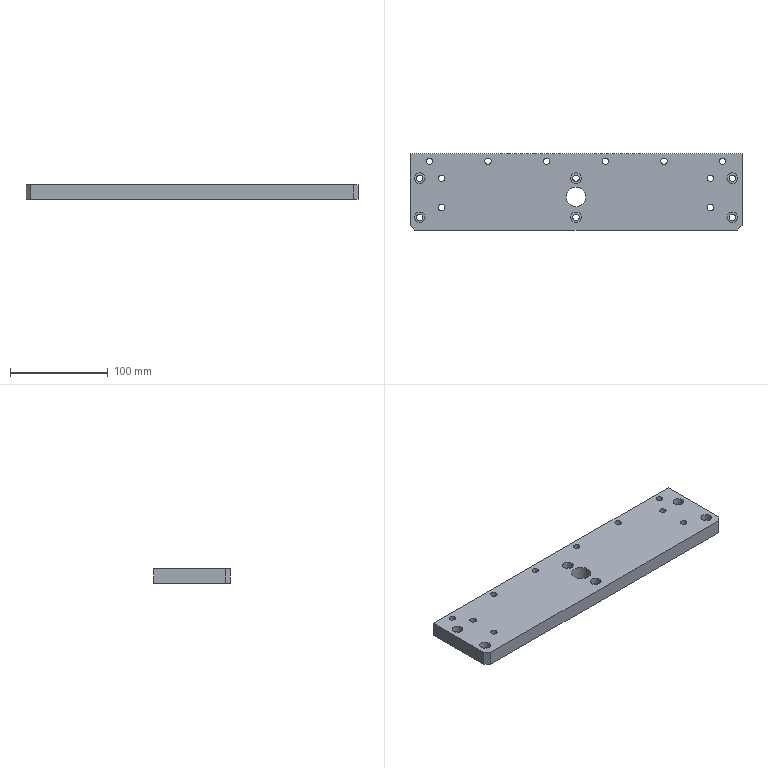Part | NX | 1 solid | 57 faces | box 340 x 78 x 15 mm | volume 377884 mm3 | cylinder 33 | plane 24 | commonest cylinder face diameters 6.6 x16 11 x16 20 x1
STEP:
#1=CARTESIAN_POINT('',(170.,-34.,7.5));
#2=VERTEX_POINT('',#1);
#3=CARTESIAN_POINT('',(170.,39.,7.5));
#4=VERTEX_POINT('',#3);
#5=CARTESIAN_POINT('',(170.,39.,7.5));
#6=DIRECTION('',(0.,1.,0.));
#7=VECTOR('',#6,1000.);
#8=LINE('',#5,#7);
#9=EDGE_CURVE('',#2,#4,#8,.T.);
#10=ORIENTED_EDGE('',*,*,#9,.F.);
#11=CARTESIAN_POINT('',(170.,-34.,-7.5));
#12=VERTEX_POINT('',#11);
#13=CARTESIAN_POINT('',(170.,-34.,7.5));
#14=DIRECTION('',(0.,0.,-1.));
#15=VECTOR('',#14,1000.);
#16=LINE('',#13,#15);
#17=EDGE_CURVE('',#2,#12,#16,.T.);
#18=ORIENTED_EDGE('',*,*,#17,.T.);
#19=CARTESIAN_POINT('',(170.,39.,-7.5));
#20=VERTEX_POINT('',#19);
#21=CARTESIAN_POINT('',(170.,39.,-7.5));
#22=DIRECTION('',(0.,1.,0.));
#23=VECTOR('',#22,1000.);
#24=LINE('',#21,#23);
#25=EDGE_CURVE('',#12,#20,#24,.T.);
#26=ORIENTED_EDGE('',*,*,#25,.T.);
#27=CARTESIAN_POINT('',(170.,39.,7.5));
#28=DIRECTION('',(0.,0.,-1.));
#29=VECTOR('',#28,1000.);
#30=LINE('',#27,#29);
#31=EDGE_CURVE('',#4,#20,#30,.T.);
#32=ORIENTED_EDGE('',*,*,#31,.F.);
#33=EDGE_LOOP('',(#10,#18,#26,#32));
#34=FACE_BOUND('',#33,.T.);
#35=CARTESIAN_POINT('',(170.,39.,7.5));
#36=DIRECTION('',(-1.,0.,0.));
#37=DIRECTION('',(0.,-1.,0.));
#38=AXIS2_PLACEMENT_3D('',#35,#36,#37);
#39=PLANE('',#38);
#40=ADVANCED_FACE('',(#34),#39,.F.);
#41=CARTESIAN_POINT('',(-170.,39.,-7.5));
#42=VERTEX_POINT('',#41);
#43=CARTESIAN_POINT('',(-170.,39.,-7.5));
#44=DIRECTION('',(-1.,0.,0.));
#45=VECTOR('',#44,1000.);
#46=LINE('',#43,#45);
#47=EDGE_CURVE('',#20,#42,#46,.T.);
#48=ORIENTED_EDGE('',*,*,#47,.T.);
#49=CARTESIAN_POINT('',(-170.,39.,7.5));
#50=VERTEX_POINT('',#49);
#51=CARTESIAN_POINT('',(-170.,39.,7.5));
#52=DIRECTION('',(0.,0.,-1.));
#53=VECTOR('',#52,1000.);
#54=LINE('',#51,#53);
#55=EDGE_CURVE('',#50,#42,#54,.T.);
#56=ORIENTED_EDGE('',*,*,#55,.F.);
#57=CARTESIAN_POINT('',(-170.,39.,7.5));
#58=DIRECTION('',(-1.,0.,0.));
#59=VECTOR('',#58,1000.);
#60=LINE('',#57,#59);
#61=EDGE_CURVE('',#4,#50,#60,.T.);
#62=ORIENTED_EDGE('',*,*,#61,.F.);
#63=ORIENTED_EDGE('',*,*,#31,.T.);
#64=EDGE_LOOP('',(#48,#56,#62,#63));
#65=FACE_BOUND('',#64,.T.);
#66=CARTESIAN_POINT('',(-170.,39.,7.5));
#67=DIRECTION('',(0.,-1.,0.));
#68=DIRECTION('',(0.,0.,-1.));
#69=AXIS2_PLACEMENT_3D('',#66,#67,#68);
#70=PLANE('',#69);
#71=ADVANCED_FACE('',(#65),#70,.F.);
#72=CARTESIAN_POINT('',(-170.,-34.,-7.5));
#73=VERTEX_POINT('',#72);
#74=CARTESIAN_POINT('',(-170.,39.,-7.5));
#75=DIRECTION('',(0.,-1.,0.));
#76=VECTOR('',#75,1000.);
#77=LINE('',#74,#76);
#78=EDGE_CURVE('',#42,#73,#77,.T.);
#79=ORIENTED_EDGE('',*,*,#78,.T.);
#80=CARTESIAN_POINT('',(-170.,-34.,7.5));
#81=VERTEX_POINT('',#80);
#82=CARTESIAN_POINT('',(-170.,-34.,7.5));
#83=DIRECTION('',(0.,0.,1.));
#84=VECTOR('',#83,1000.);
#85=LINE('',#82,#84);
#86=EDGE_CURVE('',#73,#81,#85,.T.);
#87=ORIENTED_EDGE('',*,*,#86,.T.);
#88=CARTESIAN_POINT('',(-170.,39.,7.5));
#89=DIRECTION('',(0.,-1.,0.));
#90=VECTOR('',#89,1000.);
#91=LINE('',#88,#90);
#92=EDGE_CURVE('',#50,#81,#91,.T.);
#93=ORIENTED_EDGE('',*,*,#92,.F.);
#94=ORIENTED_EDGE('',*,*,#55,.T.);
#95=EDGE_LOOP('',(#79,#87,#93,#94));
#96=FACE_BOUND('',#95,.T.);
#97=CARTESIAN_POINT('',(-170.,39.,7.5));
#98=DIRECTION('',(1.,0.,0.));
#99=DIRECTION('',(0.,0.,-1.));
#100=AXIS2_PLACEMENT_3D('',#97,#98,#99);
#101=PLANE('',#100);
#102=ADVANCED_FACE('',(#96),#101,.F.);
#103=CARTESIAN_POINT('',(-165.,-39.,-7.5));
#104=VERTEX_POINT('',#103);
#105=CARTESIAN_POINT('',(165.,-39.,-7.5));
#106=VERTEX_POINT('',#105);
#107=CARTESIAN_POINT('',(-170.,-39.,-7.5));
#108=DIRECTION('',(1.,0.,0.));
#109=VECTOR('',#108,1000.);
#110=LINE('',#107,#109);
#111=EDGE_CURVE('',#104,#106,#110,.T.);
#112=ORIENTED_EDGE('',*,*,#111,.T.);
#113=CARTESIAN_POINT('',(165.,-39.,7.5));
#114=VERTEX_POINT('',#113);
#115=CARTESIAN_POINT('',(165.,-39.,7.5));
#116=DIRECTION('',(0.,0.,1.));
#117=VECTOR('',#116,1000.);
#118=LINE('',#115,#117);
#119=EDGE_CURVE('',#106,#114,#118,.T.);
#120=ORIENTED_EDGE('',*,*,#119,.T.);
#121=CARTESIAN_POINT('',(-165.,-39.,7.5));
#122=VERTEX_POINT('',#121);
#123=CARTESIAN_POINT('',(-170.,-39.,7.5));
#124=DIRECTION('',(1.,0.,0.));
#125=VECTOR('',#124,1000.);
#126=LINE('',#123,#125);
#127=EDGE_CURVE('',#122,#114,#126,.T.);
#128=ORIENTED_EDGE('',*,*,#127,.F.);
#129=CARTESIAN_POINT('',(-165.,-39.,7.5));
#130=DIRECTION('',(0.,0.,-1.));
#131=VECTOR('',#130,1000.);
#132=LINE('',#129,#131);
#133=EDGE_CURVE('',#122,#104,#132,.T.);
#134=ORIENTED_EDGE('',*,*,#133,.T.);
#135=EDGE_LOOP('',(#112,#120,#128,#134));
#136=FACE_BOUND('',#135,.T.);
#137=CARTESIAN_POINT('',(-170.,-39.,7.5));
#138=DIRECTION('',(0.,1.,0.));
#139=DIRECTION('',(0.,0.,1.));
#140=AXIS2_PLACEMENT_3D('',#137,#138,#139);
#141=PLANE('',#140);
#142=ADVANCED_FACE('',(#136),#141,.F.);
#143=CARTESIAN_POINT('',(10.,-5.,7.5));
#144=VERTEX_POINT('',#143);
#145=CARTESIAN_POINT('',(0.,-5.,7.5));
#146=DIRECTION('',(0.,0.,1.));
#147=DIRECTION('',(1.,0.,0.));
#148=AXIS2_PLACEMENT_3D('',#145,#146,#147);
#149=CIRCLE('',#148,10.);
#150=EDGE_CURVE('',#144,#144,#149,.T.);
#151=ORIENTED_EDGE('',*,*,#150,.F.);
#152=EDGE_LOOP('',(#151));
#153=FACE_BOUND('',#152,.T.);
#154=CARTESIAN_POINT('',(165.5,-26.,7.5));
#155=VERTEX_POINT('',#154);
#156=CARTESIAN_POINT('',(160.,-26.,7.5));
#157=DIRECTION('',(0.,0.,1.));
#158=DIRECTION('',(1.,0.,0.));
#159=AXIS2_PLACEMENT_3D('',#156,#157,#158);
#160=CIRCLE('',#159,5.5);
#161=EDGE_CURVE('',#155,#155,#160,.T.);
#162=ORIENTED_EDGE('',*,*,#161,.F.);
#163=EDGE_LOOP('',(#162));
#164=FACE_BOUND('',#163,.T.);
#165=CARTESIAN_POINT('',(5.5,-26.,7.5));
#166=VERTEX_POINT('',#165);
#167=CARTESIAN_POINT('',(0.,-26.,7.5));
#168=DIRECTION('',(0.,0.,1.));
#169=DIRECTION('',(1.,0.,0.));
#170=AXIS2_PLACEMENT_3D('',#167,#168,#169);
#171=CIRCLE('',#170,5.5);
#172=EDGE_CURVE('',#166,#166,#171,.T.);
#173=ORIENTED_EDGE('',*,*,#172,.F.);
#174=EDGE_LOOP('',(#173));
#175=FACE_BOUND('',#174,.T.);
#176=CARTESIAN_POINT('',(-154.5,-26.,7.5));
#177=VERTEX_POINT('',#176);
#178=CARTESIAN_POINT('',(-160.,-26.,7.5));
#179=DIRECTION('',(0.,0.,1.));
#180=DIRECTION('',(1.,0.,0.));
#181=AXIS2_PLACEMENT_3D('',#178,#179,#180);
#182=CIRCLE('',#181,5.5);
#183=EDGE_CURVE('',#177,#177,#182,.T.);
#184=ORIENTED_EDGE('',*,*,#183,.F.);
#185=EDGE_LOOP('',(#184));
#186=FACE_BOUND('',#185,.T.);
#187=CARTESIAN_POINT('',(165.5,14.,7.5));
#188=VERTEX_POINT('',#187);
#189=CARTESIAN_POINT('',(160.,14.,7.5));
#190=DIRECTION('',(0.,0.,1.));
#191=DIRECTION('',(1.,0.,0.));
#192=AXIS2_PLACEMENT_3D('',#189,#190,#191);
#193=CIRCLE('',#192,5.5);
#194=EDGE_CURVE('',#188,#188,#193,.T.);
#195=ORIENTED_EDGE('',*,*,#194,.F.);
#196=EDGE_LOOP('',(#195));
#197=FACE_BOUND('',#196,.T.);
#198=CARTESIAN_POINT('',(5.5,14.,7.5));
#199=VERTEX_POINT('',#198);
#200=CARTESIAN_POINT('',(0.,14.,7.5));
#201=DIRECTION('',(0.,0.,1.));
#202=DIRECTION('',(1.,0.,0.));
#203=AXIS2_PLACEMENT_3D('',#200,#201,#202);
#204=CIRCLE('',#203,5.5);
#205=EDGE_CURVE('',#199,#199,#204,.T.);
#206=ORIENTED_EDGE('',*,*,#205,.F.);
#207=EDGE_LOOP('',(#206));
#208=FACE_BOUND('',#207,.T.);
#209=CARTESIAN_POINT('',(-154.5,14.,7.5));
#210=VERTEX_POINT('',#209);
#211=CARTESIAN_POINT('',(-160.,14.,7.5));
#212=DIRECTION('',(0.,0.,1.));
#213=DIRECTION('',(1.,0.,0.));
#214=AXIS2_PLACEMENT_3D('',#211,#212,#213);
#215=CIRCLE('',#214,5.5);
#216=EDGE_CURVE('',#210,#210,#215,.T.);
#217=ORIENTED_EDGE('',*,*,#216,.F.);
#218=EDGE_LOOP('',(#217));
#219=FACE_BOUND('',#218,.T.);
#220=CARTESIAN_POINT('',(86.7,31.5,7.5));
#221=VERTEX_POINT('',#220);
#222=CARTESIAN_POINT('',(90.,31.5,7.5));
#223=DIRECTION('',(0.,0.,-1.));
#224=DIRECTION('',(-1.,0.,0.));
#225=AXIS2_PLACEMENT_3D('',#222,#223,#224);
#226=CIRCLE('',#225,3.3);
#227=EDGE_CURVE('',#221,#221,#226,.T.);
#228=ORIENTED_EDGE('',*,*,#227,.T.);
#229=EDGE_LOOP('',(#228));
#230=FACE_BOUND('',#229,.T.);
#231=CARTESIAN_POINT('',(26.7,31.5,7.5));
#232=VERTEX_POINT('',#231);
#233=CARTESIAN_POINT('',(30.,31.5,7.5));
#234=DIRECTION('',(0.,0.,-1.));
#235=DIRECTION('',(-1.,0.,0.));
#236=AXIS2_PLACEMENT_3D('',#233,#234,#235);
#237=CIRCLE('',#236,3.3);
#238=EDGE_CURVE('',#232,#232,#237,.T.);
#239=ORIENTED_EDGE('',*,*,#238,.T.);
#240=EDGE_LOOP('',(#239));
#241=FACE_BOUND('',#240,.T.);
#242=CARTESIAN_POINT('',(-33.3,31.5,7.5));
#243=VERTEX_POINT('',#242);
#244=CARTESIAN_POINT('',(-30.,31.5,7.5));
#245=DIRECTION('',(0.,0.,-1.));
#246=DIRECTION('',(-1.,0.,0.));
#247=AXIS2_PLACEMENT_3D('',#244,#245,#246);
#248=CIRCLE('',#247,3.3);
#249=EDGE_CURVE('',#243,#243,#248,.T.);
#250=ORIENTED_EDGE('',*,*,#249,.T.);
#251=EDGE_LOOP('',(#250));
#252=FACE_BOUND('',#251,.T.);
#253=CARTESIAN_POINT('',(-93.3,31.5,7.5));
#254=VERTEX_POINT('',#253);
#255=CARTESIAN_POINT('',(-90.,31.5,7.5));
#256=DIRECTION('',(0.,0.,-1.));
#257=DIRECTION('',(-1.,0.,0.));
#258=AXIS2_PLACEMENT_3D('',#255,#256,#257);
#259=CIRCLE('',#258,3.3);
#260=EDGE_CURVE('',#254,#254,#259,.T.);
#261=ORIENTED_EDGE('',*,*,#260,.T.);
#262=EDGE_LOOP('',(#261));
#263=FACE_BOUND('',#262,.T.);
#264=CARTESIAN_POINT('',(-140.8,-16.,7.5));
#265=VERTEX_POINT('',#264);
#266=CARTESIAN_POINT('',(-137.5,-16.,7.5));
#267=DIRECTION('',(0.,0.,-1.));
#268=DIRECTION('',(-1.,0.,0.));
#269=AXIS2_PLACEMENT_3D('',#266,#267,#268);
#270=CIRCLE('',#269,3.3);
#271=EDGE_CURVE('',#265,#265,#270,.T.);
#272=ORIENTED_EDGE('',*,*,#271,.T.);
#273=EDGE_LOOP('',(#272));
#274=FACE_BOUND('',#273,.T.);
#275=CARTESIAN_POINT('',(-140.8,14.,7.5));
#276=VERTEX_POINT('',#275);
#277=CARTESIAN_POINT('',(-137.5,14.,7.5));
#278=DIRECTION('',(0.,0.,-1.));
#279=DIRECTION('',(-1.,0.,0.));
#280=AXIS2_PLACEMENT_3D('',#277,#278,#279);
#281=CIRCLE('',#280,3.3);
#282=EDGE_CURVE('',#276,#276,#281,.T.);
#283=ORIENTED_EDGE('',*,*,#282,.T.);
#284=EDGE_LOOP('',(#283));
#285=FACE_BOUND('',#284,.T.);
#286=CARTESIAN_POINT('',(134.2,-16.,7.5));
#287=VERTEX_POINT('',#286);
#288=CARTESIAN_POINT('',(137.5,-16.,7.5));
#289=DIRECTION('',(0.,0.,-1.));
#290=DIRECTION('',(-1.,0.,0.));
#291=AXIS2_PLACEMENT_3D('',#288,#289,#290);
#292=CIRCLE('',#291,3.3);
#293=EDGE_CURVE('',#287,#287,#292,.T.);
#294=ORIENTED_EDGE('',*,*,#293,.T.);
#295=EDGE_LOOP('',(#294));
#296=FACE_BOUND('',#295,.T.);
#297=CARTESIAN_POINT('',(134.2,14.,7.5));
#298=VERTEX_POINT('',#297);
#299=CARTESIAN_POINT('',(137.5,14.,7.5));
#300=DIRECTION('',(0.,0.,-1.));
#301=DIRECTION('',(-1.,0.,0.));
#302=AXIS2_PLACEMENT_3D('',#299,#300,#301);
#303=CIRCLE('',#302,3.3);
#304=EDGE_CURVE('',#298,#298,#303,.T.);
#305=ORIENTED_EDGE('',*,*,#304,.T.);
#306=EDGE_LOOP('',(#305));
#307=FACE_BOUND('',#306,.T.);
#308=CARTESIAN_POINT('',(146.7,31.5,7.5));
#309=VERTEX_POINT('',#308);
#310=CARTESIAN_POINT('',(150.,31.5,7.5));
#311=DIRECTION('',(0.,0.,-1.));
#312=DIRECTION('',(-1.,0.,0.));
#313=AXIS2_PLACEMENT_3D('',#310,#311,#312);
#314=CIRCLE('',#313,3.3);
#315=EDGE_CURVE('',#309,#309,#314,.T.);
#316=ORIENTED_EDGE('',*,*,#315,.T.);
#317=EDGE_LOOP('',(#316));
#318=FACE_BOUND('',#317,.T.);
#319=CARTESIAN_POINT('',(-153.3,31.5,7.5));
#320=VERTEX_POINT('',#319);
#321=CARTESIAN_POINT('',(-150.,31.5,7.5));
#322=DIRECTION('',(0.,0.,-1.));
#323=DIRECTION('',(-1.,0.,0.));
#324=AXIS2_PLACEMENT_3D('',#321,#322,#323);
#325=CIRCLE('',#324,3.3);
#326=EDGE_CURVE('',#320,#320,#325,.T.);
#327=ORIENTED_EDGE('',*,*,#326,.T.);
#328=EDGE_LOOP('',(#327));
#329=FACE_BOUND('',#328,.T.);
#330=ORIENTED_EDGE('',*,*,#127,.T.);
#331=CARTESIAN_POINT('',(102.,-102.,7.5));
#332=DIRECTION('',(-0.7071,-0.7071,0.));
#333=VECTOR('',#332,1000.);
#334=LINE('',#331,#333);
#335=EDGE_CURVE('',#114,#2,#334,.F.);
#336=ORIENTED_EDGE('',*,*,#335,.T.);
#337=ORIENTED_EDGE('',*,*,#9,.T.);
#338=ORIENTED_EDGE('',*,*,#61,.T.);
#339=ORIENTED_EDGE('',*,*,#92,.T.);
#340=CARTESIAN_POINT('',(-102.,-102.,7.5));
#341=DIRECTION('',(-0.7071,0.7071,0.));
#342=VECTOR('',#341,1000.);
#343=LINE('',#340,#342);
#344=EDGE_CURVE('',#81,#122,#343,.F.);
#345=ORIENTED_EDGE('',*,*,#344,.T.);
#346=EDGE_LOOP('',(#330,#336,#337,#338,#339,#345));
#347=FACE_BOUND('',#346,.T.);
#348=CARTESIAN_POINT('',(0.,0.,7.5));
#349=DIRECTION('',(0.,0.,1.));
#350=DIRECTION('',(1.,0.,0.));
#351=AXIS2_PLACEMENT_3D('',#348,#349,#350);
#352=PLANE('',#351);
#353=ADVANCED_FACE('',(#153,#164,#175,#186,#197,#208,#219,#230,#241,#252,#263,#274,#285,#296,#307,#318,#329,#347),#352,.T.);
#354=CARTESIAN_POINT('',(10.,-5.,-7.5));
#355=VERTEX_POINT('',#354);
#356=CARTESIAN_POINT('',(0.,-5.,-7.5));
#357=DIRECTION('',(0.,0.,1.));
#358=DIRECTION('',(1.,0.,0.));
#359=AXIS2_PLACEMENT_3D('',#356,#357,#358);
#360=CIRCLE('',#359,10.);
#361=EDGE_CURVE('',#355,#355,#360,.T.);
#362=ORIENTED_EDGE('',*,*,#361,.T.);
#363=EDGE_LOOP('',(#362));
#364=FACE_BOUND('',#363,.T.);
#365=CARTESIAN_POINT('',(163.3,-26.,-7.5));
#366=VERTEX_POINT('',#365);
#367=CARTESIAN_POINT('',(160.,-26.,-7.5));
#368=DIRECTION('',(0.,0.,1.));
#369=DIRECTION('',(1.,0.,0.));
#370=AXIS2_PLACEMENT_3D('',#367,#368,#369);
#371=CIRCLE('',#370,3.3);
#372=EDGE_CURVE('',#366,#366,#371,.T.);
#373=ORIENTED_EDGE('',*,*,#372,.T.);
#374=EDGE_LOOP('',(#373));
#375=FACE_BOUND('',#374,.T.);
#376=CARTESIAN_POINT('',(3.3,-26.,-7.5));
#377=VERTEX_POINT('',#376);
#378=CARTESIAN_POINT('',(0.,-26.,-7.5));
#379=DIRECTION('',(0.,0.,1.));
#380=DIRECTION('',(1.,0.,0.));
#381=AXIS2_PLACEMENT_3D('',#378,#379,#380);
#382=CIRCLE('',#381,3.3);
#383=EDGE_CURVE('',#377,#377,#382,.T.);
#384=ORIENTED_EDGE('',*,*,#383,.T.);
#385=EDGE_LOOP('',(#384));
#386=FACE_BOUND('',#385,.T.);
#387=CARTESIAN_POINT('',(-156.7,-26.,-7.5));
#388=VERTEX_POINT('',#387);
#389=CARTESIAN_POINT('',(-160.,-26.,-7.5));
#390=DIRECTION('',(0.,0.,1.));
#391=DIRECTION('',(1.,0.,0.));
#392=AXIS2_PLACEMENT_3D('',#389,#390,#391);
#393=CIRCLE('',#392,3.3);
#394=EDGE_CURVE('',#388,#388,#393,.T.);
#395=ORIENTED_EDGE('',*,*,#394,.T.);
#396=EDGE_LOOP('',(#395));
#397=FACE_BOUND('',#396,.T.);
#398=CARTESIAN_POINT('',(163.3,14.,-7.5));
#399=VERTEX_POINT('',#398);
#400=CARTESIAN_POINT('',(160.,14.,-7.5));
#401=DIRECTION('',(0.,0.,1.));
#402=DIRECTION('',(1.,0.,0.));
#403=AXIS2_PLACEMENT_3D('',#400,#401,#402);
#404=CIRCLE('',#403,3.3);
#405=EDGE_CURVE('',#399,#399,#404,.T.);
#406=ORIENTED_EDGE('',*,*,#405,.T.);
#407=EDGE_LOOP('',(#406));
#408=FACE_BOUND('',#407,.T.);
#409=CARTESIAN_POINT('',(3.3,14.,-7.5));
#410=VERTEX_POINT('',#409);
#411=CARTESIAN_POINT('',(0.,14.,-7.5));
#412=DIRECTION('',(0.,0.,1.));
#413=DIRECTION('',(1.,0.,0.));
#414=AXIS2_PLACEMENT_3D('',#411,#412,#413);
#415=CIRCLE('',#414,3.3);
#416=EDGE_CURVE('',#410,#410,#415,.T.);
#417=ORIENTED_EDGE('',*,*,#416,.T.);
#418=EDGE_LOOP('',(#417));
#419=FACE_BOUND('',#418,.T.);
#420=CARTESIAN_POINT('',(-156.7,14.,-7.5));
#421=VERTEX_POINT('',#420);
#422=CARTESIAN_POINT('',(-160.,14.,-7.5));
#423=DIRECTION('',(0.,0.,1.));
#424=DIRECTION('',(1.,0.,0.));
#425=AXIS2_PLACEMENT_3D('',#422,#423,#424);
#426=CIRCLE('',#425,3.3);
#427=EDGE_CURVE('',#421,#421,#426,.T.);
#428=ORIENTED_EDGE('',*,*,#427,.T.);
#429=EDGE_LOOP('',(#428));
#430=FACE_BOUND('',#429,.T.);
#431=CARTESIAN_POINT('',(84.5,31.5,-7.5));
#432=VERTEX_POINT('',#431);
#433=CARTESIAN_POINT('',(90.,31.5,-7.5));
#434=DIRECTION('',(0.,0.,-1.));
#435=DIRECTION('',(-1.,0.,0.));
#436=AXIS2_PLACEMENT_3D('',#433,#434,#435);
#437=CIRCLE('',#436,5.5);
#438=EDGE_CURVE('',#432,#432,#437,.T.);
#439=ORIENTED_EDGE('',*,*,#438,.F.);
#440=EDGE_LOOP('',(#439));
#441=FACE_BOUND('',#440,.T.);
#442=CARTESIAN_POINT('',(24.5,31.5,-7.5));
#443=VERTEX_POINT('',#442);
#444=CARTESIAN_POINT('',(30.,31.5,-7.5));
#445=DIRECTION('',(0.,0.,-1.));
#446=DIRECTION('',(-1.,0.,0.));
#447=AXIS2_PLACEMENT_3D('',#444,#445,#446);
#448=CIRCLE('',#447,5.5);
#449=EDGE_CURVE('',#443,#443,#448,.T.);
#450=ORIENTED_EDGE('',*,*,#449,.F.);
#451=EDGE_LOOP('',(#450));
#452=FACE_BOUND('',#451,.T.);
#453=CARTESIAN_POINT('',(-35.5,31.5,-7.5));
#454=VERTEX_POINT('',#453);
#455=CARTESIAN_POINT('',(-30.,31.5,-7.5));
#456=DIRECTION('',(0.,0.,-1.));
#457=DIRECTION('',(-1.,0.,0.));
#458=AXIS2_PLACEMENT_3D('',#455,#456,#457);
#459=CIRCLE('',#458,5.5);
#460=EDGE_CURVE('',#454,#454,#459,.T.);
#461=ORIENTED_EDGE('',*,*,#460,.F.);
#462=EDGE_LOOP('',(#461));
#463=FACE_BOUND('',#462,.T.);
#464=CARTESIAN_POINT('',(-95.5,31.5,-7.5));
#465=VERTEX_POINT('',#464);
#466=CARTESIAN_POINT('',(-90.,31.5,-7.5));
#467=DIRECTION('',(0.,0.,-1.));
#468=DIRECTION('',(-1.,0.,0.));
#469=AXIS2_PLACEMENT_3D('',#466,#467,#468);
#470=CIRCLE('',#469,5.5);
#471=EDGE_CURVE('',#465,#465,#470,.T.);
#472=ORIENTED_EDGE('',*,*,#471,.F.);
#473=EDGE_LOOP('',(#472));
#474=FACE_BOUND('',#473,.T.);
#475=CARTESIAN_POINT('',(-143.,-16.,-7.5));
#476=VERTEX_POINT('',#475);
#477=CARTESIAN_POINT('',(-137.5,-16.,-7.5));
#478=DIRECTION('',(0.,0.,-1.));
#479=DIRECTION('',(-1.,0.,0.));
#480=AXIS2_PLACEMENT_3D('',#477,#478,#479);
#481=CIRCLE('',#480,5.5);
#482=EDGE_CURVE('',#476,#476,#481,.T.);
#483=ORIENTED_EDGE('',*,*,#482,.F.);
#484=EDGE_LOOP('',(#483));
#485=FACE_BOUND('',#484,.T.);
#486=CARTESIAN_POINT('',(-143.,14.,-7.5));
#487=VERTEX_POINT('',#486);
#488=CARTESIAN_POINT('',(-137.5,14.,-7.5));
#489=DIRECTION('',(0.,0.,-1.));
#490=DIRECTION('',(-1.,0.,0.));
#491=AXIS2_PLACEMENT_3D('',#488,#489,#490);
#492=CIRCLE('',#491,5.5);
#493=EDGE_CURVE('',#487,#487,#492,.T.);
#494=ORIENTED_EDGE('',*,*,#493,.F.);
#495=EDGE_LOOP('',(#494));
#496=FACE_BOUND('',#495,.T.);
#497=CARTESIAN_POINT('',(132.,-16.,-7.5));
#498=VERTEX_POINT('',#497);
#499=CARTESIAN_POINT('',(137.5,-16.,-7.5));
#500=DIRECTION('',(0.,0.,-1.));
#501=DIRECTION('',(-1.,0.,0.));
#502=AXIS2_PLACEMENT_3D('',#499,#500,#501);
#503=CIRCLE('',#502,5.5);
#504=EDGE_CURVE('',#498,#498,#503,.T.);
#505=ORIENTED_EDGE('',*,*,#504,.F.);
#506=EDGE_LOOP('',(#505));
#507=FACE_BOUND('',#506,.T.);
#508=CARTESIAN_POINT('',(132.,14.,-7.5));
#509=VERTEX_POINT('',#508);
#510=CARTESIAN_POINT('',(137.5,14.,-7.5));
#511=DIRECTION('',(0.,0.,-1.));
#512=DIRECTION('',(-1.,0.,0.));
#513=AXIS2_PLACEMENT_3D('',#510,#511,#512);
#514=CIRCLE('',#513,5.5);
#515=EDGE_CURVE('',#509,#509,#514,.T.);
#516=ORIENTED_EDGE('',*,*,#515,.F.);
#517=EDGE_LOOP('',(#516));
#518=FACE_BOUND('',#517,.T.);
#519=CARTESIAN_POINT('',(144.5,31.5,-7.5));
#520=VERTEX_POINT('',#519);
#521=CARTESIAN_POINT('',(150.,31.5,-7.5));
#522=DIRECTION('',(0.,0.,-1.));
#523=DIRECTION('',(-1.,0.,0.));
#524=AXIS2_PLACEMENT_3D('',#521,#522,#523);
#525=CIRCLE('',#524,5.5);
#526=EDGE_CURVE('',#520,#520,#525,.T.);
#527=ORIENTED_EDGE('',*,*,#526,.F.);
#528=EDGE_LOOP('',(#527));
#529=FACE_BOUND('',#528,.T.);
#530=CARTESIAN_POINT('',(-155.5,31.5,-7.5));
#531=VERTEX_POINT('',#530);
#532=CARTESIAN_POINT('',(-150.,31.5,-7.5));
#533=DIRECTION('',(0.,0.,-1.));
#534=DIRECTION('',(-1.,0.,0.));
#535=AXIS2_PLACEMENT_3D('',#532,#533,#534);
#536=CIRCLE('',#535,5.5);
#537=EDGE_CURVE('',#531,#531,#536,.T.);
#538=ORIENTED_EDGE('',*,*,#537,.F.);
#539=EDGE_LOOP('',(#538));
#540=FACE_BOUND('',#539,.T.);
#541=ORIENTED_EDGE('',*,*,#25,.F.);
#542=CARTESIAN_POINT('',(170.,-34.,-7.5));
#543=DIRECTION('',(0.7071,0.7071,0.));
#544=VECTOR('',#543,1000.);
#545=LINE('',#542,#544);
#546=EDGE_CURVE('',#12,#106,#545,.F.);
#547=ORIENTED_EDGE('',*,*,#546,.T.);
#548=ORIENTED_EDGE('',*,*,#111,.F.);
#549=CARTESIAN_POINT('',(-165.,-39.,-7.5));
#550=DIRECTION('',(0.7071,-0.7071,0.));
#551=VECTOR('',#550,1000.);
#552=LINE('',#549,#551);
#553=EDGE_CURVE('',#104,#73,#552,.F.);
#554=ORIENTED_EDGE('',*,*,#553,.T.);
#555=ORIENTED_EDGE('',*,*,#78,.F.);
#556=ORIENTED_EDGE('',*,*,#47,.F.);
#557=EDGE_LOOP('',(#541,#547,#548,#554,#555,#556));
#558=FACE_BOUND('',#557,.T.);
#559=CARTESIAN_POINT('',(0.,0.,-7.5));
#560=DIRECTION('',(0.,0.,1.));
#561=DIRECTION('',(1.,0.,0.));
#562=AXIS2_PLACEMENT_3D('',#559,#560,#561);
#563=PLANE('',#562);
#564=ADVANCED_FACE('',(#364,#375,#386,#397,#408,#419,#430,#441,#452,#463,#474,#485,#496,#507,#518,#529,#540,#558),#563,.F.);
#565=ORIENTED_EDGE('',*,*,#326,.F.);
#566=EDGE_LOOP('',(#565));
#567=FACE_BOUND('',#566,.T.);
#568=CARTESIAN_POINT('',(-153.3,31.5,-0.7));
#569=VERTEX_POINT('',#568);
#570=CARTESIAN_POINT('',(-150.,31.5,-0.7));
#571=DIRECTION('',(0.,0.,-1.));
#572=DIRECTION('',(-1.,0.,0.));
#573=AXIS2_PLACEMENT_3D('',#570,#571,#572);
#574=CIRCLE('',#573,3.3);
#575=EDGE_CURVE('',#569,#569,#574,.T.);
#576=ORIENTED_EDGE('',*,*,#575,.T.);
#577=EDGE_LOOP('',(#576));
#578=FACE_BOUND('',#577,.T.);
#579=CARTESIAN_POINT('',(-150.,31.5,-7.5));
#580=DIRECTION('',(0.,0.,-1.));
#581=DIRECTION('',(-1.,0.,0.));
#582=AXIS2_PLACEMENT_3D('',#579,#580,#581);
#583=CYLINDRICAL_SURFACE('',#582,3.3);
#584=ADVANCED_FACE('',(#567,#578),#583,.F.);
#585=ORIENTED_EDGE('',*,*,#575,.F.);
#586=EDGE_LOOP('',(#585));
#587=FACE_BOUND('',#586,.T.);
#588=CARTESIAN_POINT('',(-155.5,31.5,-0.7));
#589=VERTEX_POINT('',#588);
#590=CARTESIAN_POINT('',(-150.,31.5,-0.7));
#591=DIRECTION('',(0.,0.,-1.));
#592=DIRECTION('',(-1.,0.,0.));
#593=AXIS2_PLACEMENT_3D('',#590,#591,#592);
#594=CIRCLE('',#593,5.5);
#595=EDGE_CURVE('',#589,#589,#594,.T.);
#596=ORIENTED_EDGE('',*,*,#595,.T.);
#597=EDGE_LOOP('',(#596));
#598=FACE_BOUND('',#597,.T.);
#599=CARTESIAN_POINT('',(-146.7,31.5,-0.7));
#600=DIRECTION('',(0.,0.,1.));
#601=DIRECTION('',(1.,0.,0.));
#602=AXIS2_PLACEMENT_3D('',#599,#600,#601);
#603=PLANE('',#602);
#604=ADVANCED_FACE('',(#587,#598),#603,.F.);
#605=ORIENTED_EDGE('',*,*,#595,.F.);
#606=EDGE_LOOP('',(#605));
#607=FACE_BOUND('',#606,.T.);
#608=ORIENTED_EDGE('',*,*,#537,.T.);
#609=EDGE_LOOP('',(#608));
#610=FACE_BOUND('',#609,.T.);
#611=CARTESIAN_POINT('',(-150.,31.5,-7.5));
#612=DIRECTION('',(0.,0.,-1.));
#613=DIRECTION('',(-1.,0.,0.));
#614=AXIS2_PLACEMENT_3D('',#611,#612,#613);
#615=CYLINDRICAL_SURFACE('',#614,5.5);
#616=ADVANCED_FACE('',(#607,#610),#615,.F.);
#617=ORIENTED_EDGE('',*,*,#315,.F.);
#618=EDGE_LOOP('',(#617));
#619=FACE_BOUND('',#618,.T.);
#620=CARTESIAN_POINT('',(146.7,31.5,-0.7));
#621=VERTEX_POINT('',#620);
#622=CARTESIAN_POINT('',(150.,31.5,-0.7));
#623=DIRECTION('',(0.,0.,-1.));
#624=DIRECTION('',(-1.,0.,0.));
#625=AXIS2_PLACEMENT_3D('',#622,#623,#624);
#626=CIRCLE('',#625,3.3);
#627=EDGE_CURVE('',#621,#621,#626,.T.);
#628=ORIENTED_EDGE('',*,*,#627,.T.);
#629=EDGE_LOOP('',(#628));
#630=FACE_BOUND('',#629,.T.);
#631=CARTESIAN_POINT('',(150.,31.5,-7.5));
#632=DIRECTION('',(0.,0.,-1.));
#633=DIRECTION('',(-1.,0.,0.));
#634=AXIS2_PLACEMENT_3D('',#631,#632,#633);
#635=CYLINDRICAL_SURFACE('',#634,3.3);
#636=ADVANCED_FACE('',(#619,#630),#635,.F.);
#637=ORIENTED_EDGE('',*,*,#627,.F.);
#638=EDGE_LOOP('',(#637));
#639=FACE_BOUND('',#638,.T.);
#640=CARTESIAN_POINT('',(144.5,31.5,-0.7));
#641=VERTEX_POINT('',#640);
#642=CARTESIAN_POINT('',(150.,31.5,-0.7));
#643=DIRECTION('',(0.,0.,-1.));
#644=DIRECTION('',(-1.,0.,0.));
#645=AXIS2_PLACEMENT_3D('',#642,#643,#644);
#646=CIRCLE('',#645,5.5);
#647=EDGE_CURVE('',#641,#641,#646,.T.);
#648=ORIENTED_EDGE('',*,*,#647,.T.);
#649=EDGE_LOOP('',(#648));
#650=FACE_BOUND('',#649,.T.);
#651=CARTESIAN_POINT('',(153.3,31.5,-0.7));
#652=DIRECTION('',(0.,0.,1.));
#653=DIRECTION('',(1.,0.,0.));
#654=AXIS2_PLACEMENT_3D('',#651,#652,#653);
#655=PLANE('',#654);
#656=ADVANCED_FACE('',(#639,#650),#655,.F.);
#657=ORIENTED_EDGE('',*,*,#647,.F.);
#658=EDGE_LOOP('',(#657));
#659=FACE_BOUND('',#658,.T.);
#660=ORIENTED_EDGE('',*,*,#526,.T.);
#661=EDGE_LOOP('',(#660));
#662=FACE_BOUND('',#661,.T.);
#663=CARTESIAN_POINT('',(150.,31.5,-7.5));
#664=DIRECTION('',(0.,0.,-1.));
#665=DIRECTION('',(-1.,0.,0.));
#666=AXIS2_PLACEMENT_3D('',#663,#664,#665);
#667=CYLINDRICAL_SURFACE('',#666,5.5);
#668=ADVANCED_FACE('',(#659,#662),#667,.F.);
#669=ORIENTED_EDGE('',*,*,#304,.F.);
#670=EDGE_LOOP('',(#669));
#671=FACE_BOUND('',#670,.T.);
#672=CARTESIAN_POINT('',(134.2,14.,-0.7));
#673=VERTEX_POINT('',#672);
#674=CARTESIAN_POINT('',(137.5,14.,-0.7));
#675=DIRECTION('',(0.,0.,-1.));
#676=DIRECTION('',(-1.,0.,0.));
#677=AXIS2_PLACEMENT_3D('',#674,#675,#676);
#678=CIRCLE('',#677,3.3);
#679=EDGE_CURVE('',#673,#673,#678,.T.);
#680=ORIENTED_EDGE('',*,*,#679,.T.);
#681=EDGE_LOOP('',(#680));
#682=FACE_BOUND('',#681,.T.);
#683=CARTESIAN_POINT('',(137.5,14.,-7.5));
#684=DIRECTION('',(0.,0.,-1.));
#685=DIRECTION('',(-1.,0.,0.));
#686=AXIS2_PLACEMENT_3D('',#683,#684,#685);
#687=CYLINDRICAL_SURFACE('',#686,3.3);
#688=ADVANCED_FACE('',(#671,#682),#687,.F.);
#689=ORIENTED_EDGE('',*,*,#679,.F.);
#690=EDGE_LOOP('',(#689));
#691=FACE_BOUND('',#690,.T.);
#692=CARTESIAN_POINT('',(132.,14.,-0.7));
#693=VERTEX_POINT('',#692);
#694=CARTESIAN_POINT('',(137.5,14.,-0.7));
#695=DIRECTION('',(0.,0.,-1.));
#696=DIRECTION('',(-1.,0.,0.));
#697=AXIS2_PLACEMENT_3D('',#694,#695,#696);
#698=CIRCLE('',#697,5.5);
#699=EDGE_CURVE('',#693,#693,#698,.T.);
#700=ORIENTED_EDGE('',*,*,#699,.T.);
#701=EDGE_LOOP('',(#700));
#702=FACE_BOUND('',#701,.T.);
#703=CARTESIAN_POINT('',(140.8,14.,-0.7));
#704=DIRECTION('',(0.,0.,1.));
#705=DIRECTION('',(1.,0.,0.));
#706=AXIS2_PLACEMENT_3D('',#703,#704,#705);
#707=PLANE('',#706);
#708=ADVANCED_FACE('',(#691,#702),#707,.F.);
#709=ORIENTED_EDGE('',*,*,#699,.F.);
#710=EDGE_LOOP('',(#709));
#711=FACE_BOUND('',#710,.T.);
#712=ORIENTED_EDGE('',*,*,#515,.T.);
#713=EDGE_LOOP('',(#712));
#714=FACE_BOUND('',#713,.T.);
#715=CARTESIAN_POINT('',(137.5,14.,-7.5));
#716=DIRECTION('',(0.,0.,-1.));
#717=DIRECTION('',(-1.,0.,0.));
#718=AXIS2_PLACEMENT_3D('',#715,#716,#717);
#719=CYLINDRICAL_SURFACE('',#718,5.5);
#720=ADVANCED_FACE('',(#711,#714),#719,.F.);
#721=ORIENTED_EDGE('',*,*,#293,.F.);
#722=EDGE_LOOP('',(#721));
#723=FACE_BOUND('',#722,.T.);
#724=CARTESIAN_POINT('',(134.2,-16.,-0.7));
#725=VERTEX_POINT('',#724);
#726=CARTESIAN_POINT('',(137.5,-16.,-0.7));
#727=DIRECTION('',(0.,0.,-1.));
#728=DIRECTION('',(-1.,0.,0.));
#729=AXIS2_PLACEMENT_3D('',#726,#727,#728);
#730=CIRCLE('',#729,3.3);
#731=EDGE_CURVE('',#725,#725,#730,.T.);
#732=ORIENTED_EDGE('',*,*,#731,.T.);
#733=EDGE_LOOP('',(#732));
#734=FACE_BOUND('',#733,.T.);
#735=CARTESIAN_POINT('',(137.5,-16.,-7.5));
#736=DIRECTION('',(0.,0.,-1.));
#737=DIRECTION('',(-1.,0.,0.));
#738=AXIS2_PLACEMENT_3D('',#735,#736,#737);
#739=CYLINDRICAL_SURFACE('',#738,3.3);
#740=ADVANCED_FACE('',(#723,#734),#739,.F.);
#741=ORIENTED_EDGE('',*,*,#731,.F.);
#742=EDGE_LOOP('',(#741));
#743=FACE_BOUND('',#742,.T.);
#744=CARTESIAN_POINT('',(132.,-16.,-0.7));
#745=VERTEX_POINT('',#744);
#746=CARTESIAN_POINT('',(137.5,-16.,-0.7));
#747=DIRECTION('',(0.,0.,-1.));
#748=DIRECTION('',(-1.,0.,0.));
#749=AXIS2_PLACEMENT_3D('',#746,#747,#748);
#750=CIRCLE('',#749,5.5);
#751=EDGE_CURVE('',#745,#745,#750,.T.);
#752=ORIENTED_EDGE('',*,*,#751,.T.);
#753=EDGE_LOOP('',(#752));
#754=FACE_BOUND('',#753,.T.);
#755=CARTESIAN_POINT('',(140.8,-16.,-0.7));
#756=DIRECTION('',(0.,0.,1.));
#757=DIRECTION('',(1.,0.,0.));
#758=AXIS2_PLACEMENT_3D('',#755,#756,#757);
#759=PLANE('',#758);
#760=ADVANCED_FACE('',(#743,#754),#759,.F.);
#761=ORIENTED_EDGE('',*,*,#751,.F.);
#762=EDGE_LOOP('',(#761));
#763=FACE_BOUND('',#762,.T.);
#764=ORIENTED_EDGE('',*,*,#504,.T.);
#765=EDGE_LOOP('',(#764));
#766=FACE_BOUND('',#765,.T.);
#767=CARTESIAN_POINT('',(137.5,-16.,-7.5));
#768=DIRECTION('',(0.,0.,-1.));
#769=DIRECTION('',(-1.,0.,0.));
#770=AXIS2_PLACEMENT_3D('',#767,#768,#769);
#771=CYLINDRICAL_SURFACE('',#770,5.5);
#772=ADVANCED_FACE('',(#763,#766),#771,.F.);
#773=ORIENTED_EDGE('',*,*,#282,.F.);
#774=EDGE_LOOP('',(#773));
#775=FACE_BOUND('',#774,.T.);
#776=CARTESIAN_POINT('',(-140.8,14.,-0.7));
#777=VERTEX_POINT('',#776);
#778=CARTESIAN_POINT('',(-137.5,14.,-0.7));
#779=DIRECTION('',(0.,0.,-1.));
#780=DIRECTION('',(-1.,0.,0.));
#781=AXIS2_PLACEMENT_3D('',#778,#779,#780);
#782=CIRCLE('',#781,3.3);
#783=EDGE_CURVE('',#777,#777,#782,.T.);
#784=ORIENTED_EDGE('',*,*,#783,.T.);
#785=EDGE_LOOP('',(#784));
#786=FACE_BOUND('',#785,.T.);
#787=CARTESIAN_POINT('',(-137.5,14.,-7.5));
#788=DIRECTION('',(0.,0.,-1.));
#789=DIRECTION('',(-1.,0.,0.));
#790=AXIS2_PLACEMENT_3D('',#787,#788,#789);
#791=CYLINDRICAL_SURFACE('',#790,3.3);
#792=ADVANCED_FACE('',(#775,#786),#791,.F.);
#793=ORIENTED_EDGE('',*,*,#783,.F.);
#794=EDGE_LOOP('',(#793));
#795=FACE_BOUND('',#794,.T.);
#796=CARTESIAN_POINT('',(-143.,14.,-0.7));
#797=VERTEX_POINT('',#796);
#798=CARTESIAN_POINT('',(-137.5,14.,-0.7));
#799=DIRECTION('',(0.,0.,-1.));
#800=DIRECTION('',(-1.,0.,0.));
#801=AXIS2_PLACEMENT_3D('',#798,#799,#800);
#802=CIRCLE('',#801,5.5);
#803=EDGE_CURVE('',#797,#797,#802,.T.);
#804=ORIENTED_EDGE('',*,*,#803,.T.);
#805=EDGE_LOOP('',(#804));
#806=FACE_BOUND('',#805,.T.);
#807=CARTESIAN_POINT('',(-134.2,14.,-0.7));
#808=DIRECTION('',(0.,0.,1.));
#809=DIRECTION('',(1.,0.,0.));
#810=AXIS2_PLACEMENT_3D('',#807,#808,#809);
#811=PLANE('',#810);
#812=ADVANCED_FACE('',(#795,#806),#811,.F.);
#813=ORIENTED_EDGE('',*,*,#803,.F.);
#814=EDGE_LOOP('',(#813));
#815=FACE_BOUND('',#814,.T.);
#816=ORIENTED_EDGE('',*,*,#493,.T.);
#817=EDGE_LOOP('',(#816));
#818=FACE_BOUND('',#817,.T.);
#819=CARTESIAN_POINT('',(-137.5,14.,-7.5));
#820=DIRECTION('',(0.,0.,-1.));
#821=DIRECTION('',(-1.,0.,0.));
#822=AXIS2_PLACEMENT_3D('',#819,#820,#821);
#823=CYLINDRICAL_SURFACE('',#822,5.5);
#824=ADVANCED_FACE('',(#815,#818),#823,.F.);
#825=ORIENTED_EDGE('',*,*,#271,.F.);
#826=EDGE_LOOP('',(#825));
#827=FACE_BOUND('',#826,.T.);
#828=CARTESIAN_POINT('',(-140.8,-16.,-0.7));
#829=VERTEX_POINT('',#828);
#830=CARTESIAN_POINT('',(-137.5,-16.,-0.7));
#831=DIRECTION('',(0.,0.,-1.));
#832=DIRECTION('',(-1.,0.,0.));
#833=AXIS2_PLACEMENT_3D('',#830,#831,#832);
#834=CIRCLE('',#833,3.3);
#835=EDGE_CURVE('',#829,#829,#834,.T.);
#836=ORIENTED_EDGE('',*,*,#835,.T.);
#837=EDGE_LOOP('',(#836));
#838=FACE_BOUND('',#837,.T.);
#839=CARTESIAN_POINT('',(-137.5,-16.,-7.5));
#840=DIRECTION('',(0.,0.,-1.));
#841=DIRECTION('',(-1.,0.,0.));
#842=AXIS2_PLACEMENT_3D('',#839,#840,#841);
#843=CYLINDRICAL_SURFACE('',#842,3.3);
#844=ADVANCED_FACE('',(#827,#838),#843,.F.);
#845=ORIENTED_EDGE('',*,*,#835,.F.);
#846=EDGE_LOOP('',(#845));
#847=FACE_BOUND('',#846,.T.);
#848=CARTESIAN_POINT('',(-143.,-16.,-0.7));
#849=VERTEX_POINT('',#848);
#850=CARTESIAN_POINT('',(-137.5,-16.,-0.7));
#851=DIRECTION('',(0.,0.,-1.));
#852=DIRECTION('',(-1.,0.,0.));
#853=AXIS2_PLACEMENT_3D('',#850,#851,#852);
#854=CIRCLE('',#853,5.5);
#855=EDGE_CURVE('',#849,#849,#854,.T.);
#856=ORIENTED_EDGE('',*,*,#855,.T.);
#857=EDGE_LOOP('',(#856));
#858=FACE_BOUND('',#857,.T.);
#859=CARTESIAN_POINT('',(-134.2,-16.,-0.7));
#860=DIRECTION('',(0.,0.,1.));
#861=DIRECTION('',(1.,0.,0.));
#862=AXIS2_PLACEMENT_3D('',#859,#860,#861);
#863=PLANE('',#862);
#864=ADVANCED_FACE('',(#847,#858),#863,.F.);
#865=ORIENTED_EDGE('',*,*,#855,.F.);
#866=EDGE_LOOP('',(#865));
#867=FACE_BOUND('',#866,.T.);
#868=ORIENTED_EDGE('',*,*,#482,.T.);
#869=EDGE_LOOP('',(#868));
#870=FACE_BOUND('',#869,.T.);
#871=CARTESIAN_POINT('',(-137.5,-16.,-7.5));
#872=DIRECTION('',(0.,0.,-1.));
#873=DIRECTION('',(-1.,0.,0.));
#874=AXIS2_PLACEMENT_3D('',#871,#872,#873);
#875=CYLINDRICAL_SURFACE('',#874,5.5);
#876=ADVANCED_FACE('',(#867,#870),#875,.F.);
#877=ORIENTED_EDGE('',*,*,#260,.F.);
#878=EDGE_LOOP('',(#877));
#879=FACE_BOUND('',#878,.T.);
#880=CARTESIAN_POINT('',(-93.3,31.5,-0.7));
#881=VERTEX_POINT('',#880);
#882=CARTESIAN_POINT('',(-90.,31.5,-0.7));
#883=DIRECTION('',(0.,0.,-1.));
#884=DIRECTION('',(-1.,0.,0.));
#885=AXIS2_PLACEMENT_3D('',#882,#883,#884);
#886=CIRCLE('',#885,3.3);
#887=EDGE_CURVE('',#881,#881,#886,.T.);
#888=ORIENTED_EDGE('',*,*,#887,.T.);
#889=EDGE_LOOP('',(#888));
#890=FACE_BOUND('',#889,.T.);
#891=CARTESIAN_POINT('',(-90.,31.5,-7.5));
#892=DIRECTION('',(0.,0.,-1.));
#893=DIRECTION('',(-1.,0.,0.));
#894=AXIS2_PLACEMENT_3D('',#891,#892,#893);
#895=CYLINDRICAL_SURFACE('',#894,3.3);
#896=ADVANCED_FACE('',(#879,#890),#895,.F.);
#897=ORIENTED_EDGE('',*,*,#887,.F.);
#898=EDGE_LOOP('',(#897));
#899=FACE_BOUND('',#898,.T.);
#900=CARTESIAN_POINT('',(-95.5,31.5,-0.7));
#901=VERTEX_POINT('',#900);
#902=CARTESIAN_POINT('',(-90.,31.5,-0.7));
#903=DIRECTION('',(0.,0.,-1.));
#904=DIRECTION('',(-1.,0.,0.));
#905=AXIS2_PLACEMENT_3D('',#902,#903,#904);
#906=CIRCLE('',#905,5.5);
#907=EDGE_CURVE('',#901,#901,#906,.T.);
#908=ORIENTED_EDGE('',*,*,#907,.T.);
#909=EDGE_LOOP('',(#908));
#910=FACE_BOUND('',#909,.T.);
#911=CARTESIAN_POINT('',(-86.7,31.5,-0.7));
#912=DIRECTION('',(0.,0.,1.));
#913=DIRECTION('',(1.,0.,0.));
#914=AXIS2_PLACEMENT_3D('',#911,#912,#913);
#915=PLANE('',#914);
#916=ADVANCED_FACE('',(#899,#910),#915,.F.);
#917=ORIENTED_EDGE('',*,*,#907,.F.);
#918=EDGE_LOOP('',(#917));
#919=FACE_BOUND('',#918,.T.);
#920=ORIENTED_EDGE('',*,*,#471,.T.);
#921=EDGE_LOOP('',(#920));
#922=FACE_BOUND('',#921,.T.);
#923=CARTESIAN_POINT('',(-90.,31.5,-7.5));
#924=DIRECTION('',(0.,0.,-1.));
#925=DIRECTION('',(-1.,0.,0.));
#926=AXIS2_PLACEMENT_3D('',#923,#924,#925);
#927=CYLINDRICAL_SURFACE('',#926,5.5);
#928=ADVANCED_FACE('',(#919,#922),#927,.F.);
#929=ORIENTED_EDGE('',*,*,#249,.F.);
#930=EDGE_LOOP('',(#929));
#931=FACE_BOUND('',#930,.T.);
#932=CARTESIAN_POINT('',(-33.3,31.5,-0.7));
#933=VERTEX_POINT('',#932);
#934=CARTESIAN_POINT('',(-30.,31.5,-0.7));
#935=DIRECTION('',(0.,0.,-1.));
#936=DIRECTION('',(-1.,0.,0.));
#937=AXIS2_PLACEMENT_3D('',#934,#935,#936);
#938=CIRCLE('',#937,3.3);
#939=EDGE_CURVE('',#933,#933,#938,.T.);
#940=ORIENTED_EDGE('',*,*,#939,.T.);
#941=EDGE_LOOP('',(#940));
#942=FACE_BOUND('',#941,.T.);
#943=CARTESIAN_POINT('',(-30.,31.5,-7.5));
#944=DIRECTION('',(0.,0.,-1.));
#945=DIRECTION('',(-1.,0.,0.));
#946=AXIS2_PLACEMENT_3D('',#943,#944,#945);
#947=CYLINDRICAL_SURFACE('',#946,3.3);
#948=ADVANCED_FACE('',(#931,#942),#947,.F.);
#949=ORIENTED_EDGE('',*,*,#939,.F.);
#950=EDGE_LOOP('',(#949));
#951=FACE_BOUND('',#950,.T.);
#952=CARTESIAN_POINT('',(-35.5,31.5,-0.7));
#953=VERTEX_POINT('',#952);
#954=CARTESIAN_POINT('',(-30.,31.5,-0.7));
#955=DIRECTION('',(0.,0.,-1.));
#956=DIRECTION('',(-1.,0.,0.));
#957=AXIS2_PLACEMENT_3D('',#954,#955,#956);
#958=CIRCLE('',#957,5.5);
#959=EDGE_CURVE('',#953,#953,#958,.T.);
#960=ORIENTED_EDGE('',*,*,#959,.T.);
#961=EDGE_LOOP('',(#960));
#962=FACE_BOUND('',#961,.T.);
#963=CARTESIAN_POINT('',(-26.7,31.5,-0.7));
#964=DIRECTION('',(0.,0.,1.));
#965=DIRECTION('',(1.,0.,0.));
#966=AXIS2_PLACEMENT_3D('',#963,#964,#965);
#967=PLANE('',#966);
#968=ADVANCED_FACE('',(#951,#962),#967,.F.);
#969=ORIENTED_EDGE('',*,*,#959,.F.);
#970=EDGE_LOOP('',(#969));
#971=FACE_BOUND('',#970,.T.);
#972=ORIENTED_EDGE('',*,*,#460,.T.);
#973=EDGE_LOOP('',(#972));
#974=FACE_BOUND('',#973,.T.);
#975=CARTESIAN_POINT('',(-30.,31.5,-7.5));
#976=DIRECTION('',(0.,0.,-1.));
#977=DIRECTION('',(-1.,0.,0.));
#978=AXIS2_PLACEMENT_3D('',#975,#976,#977);
#979=CYLINDRICAL_SURFACE('',#978,5.5);
#980=ADVANCED_FACE('',(#971,#974),#979,.F.);
#981=ORIENTED_EDGE('',*,*,#238,.F.);
#982=EDGE_LOOP('',(#981));
#983=FACE_BOUND('',#982,.T.);
#984=CARTESIAN_POINT('',(26.7,31.5,-0.7));
#985=VERTEX_POINT('',#984);
#986=CARTESIAN_POINT('',(30.,31.5,-0.7));
#987=DIRECTION('',(0.,0.,-1.));
#988=DIRECTION('',(-1.,0.,0.));
#989=AXIS2_PLACEMENT_3D('',#986,#987,#988);
#990=CIRCLE('',#989,3.3);
#991=EDGE_CURVE('',#985,#985,#990,.T.);
#992=ORIENTED_EDGE('',*,*,#991,.T.);
#993=EDGE_LOOP('',(#992));
#994=FACE_BOUND('',#993,.T.);
#995=CARTESIAN_POINT('',(30.,31.5,-7.5));
#996=DIRECTION('',(0.,0.,-1.));
#997=DIRECTION('',(-1.,0.,0.));
#998=AXIS2_PLACEMENT_3D('',#995,#996,#997);
#999=CYLINDRICAL_SURFACE('',#998,3.3);
#1000=ADVANCED_FACE('',(#983,#994),#999,.F.);
#1001=ORIENTED_EDGE('',*,*,#991,.F.);
#1002=EDGE_LOOP('',(#1001));
#1003=FACE_BOUND('',#1002,.T.);
#1004=CARTESIAN_POINT('',(24.5,31.5,-0.7));
#1005=VERTEX_POINT('',#1004);
#1006=CARTESIAN_POINT('',(30.,31.5,-0.7));
#1007=DIRECTION('',(0.,0.,-1.));
#1008=DIRECTION('',(-1.,0.,0.));
#1009=AXIS2_PLACEMENT_3D('',#1006,#1007,#1008);
#1010=CIRCLE('',#1009,5.5);
#1011=EDGE_CURVE('',#1005,#1005,#1010,.T.);
#1012=ORIENTED_EDGE('',*,*,#1011,.T.);
#1013=EDGE_LOOP('',(#1012));
#1014=FACE_BOUND('',#1013,.T.);
#1015=CARTESIAN_POINT('',(33.3,31.5,-0.7));
#1016=DIRECTION('',(0.,0.,1.));
#1017=DIRECTION('',(1.,0.,0.));
#1018=AXIS2_PLACEMENT_3D('',#1015,#1016,#1017);
#1019=PLANE('',#1018);
#1020=ADVANCED_FACE('',(#1003,#1014),#1019,.F.);
#1021=ORIENTED_EDGE('',*,*,#1011,.F.);
#1022=EDGE_LOOP('',(#1021));
#1023=FACE_BOUND('',#1022,.T.);
#1024=ORIENTED_EDGE('',*,*,#449,.T.);
#1025=EDGE_LOOP('',(#1024));
#1026=FACE_BOUND('',#1025,.T.);
#1027=CARTESIAN_POINT('',(30.,31.5,-7.5));
#1028=DIRECTION('',(0.,0.,-1.));
#1029=DIRECTION('',(-1.,0.,0.));
#1030=AXIS2_PLACEMENT_3D('',#1027,#1028,#1029);
#1031=CYLINDRICAL_SURFACE('',#1030,5.5);
#1032=ADVANCED_FACE('',(#1023,#1026),#1031,.F.);
#1033=ORIENTED_EDGE('',*,*,#227,.F.);
#1034=EDGE_LOOP('',(#1033));
#1035=FACE_BOUND('',#1034,.T.);
#1036=CARTESIAN_POINT('',(86.7,31.5,-0.7));
#1037=VERTEX_POINT('',#1036);
#1038=CARTESIAN_POINT('',(90.,31.5,-0.7));
#1039=DIRECTION('',(0.,0.,-1.));
#1040=DIRECTION('',(-1.,0.,0.));
#1041=AXIS2_PLACEMENT_3D('',#1038,#1039,#1040);
#1042=CIRCLE('',#1041,3.3);
#1043=EDGE_CURVE('',#1037,#1037,#1042,.T.);
#1044=ORIENTED_EDGE('',*,*,#1043,.T.);
#1045=EDGE_LOOP('',(#1044));
#1046=FACE_BOUND('',#1045,.T.);
#1047=CARTESIAN_POINT('',(90.,31.5,-7.5));
#1048=DIRECTION('',(0.,0.,-1.));
#1049=DIRECTION('',(-1.,0.,0.));
#1050=AXIS2_PLACEMENT_3D('',#1047,#1048,#1049);
#1051=CYLINDRICAL_SURFACE('',#1050,3.3);
#1052=ADVANCED_FACE('',(#1035,#1046),#1051,.F.);
#1053=ORIENTED_EDGE('',*,*,#1043,.F.);
#1054=EDGE_LOOP('',(#1053));
#1055=FACE_BOUND('',#1054,.T.);
#1056=CARTESIAN_POINT('',(84.5,31.5,-0.7));
#1057=VERTEX_POINT('',#1056);
#1058=CARTESIAN_POINT('',(90.,31.5,-0.7));
#1059=DIRECTION('',(0.,0.,-1.));
#1060=DIRECTION('',(-1.,0.,0.));
#1061=AXIS2_PLACEMENT_3D('',#1058,#1059,#1060);
#1062=CIRCLE('',#1061,5.5);
#1063=EDGE_CURVE('',#1057,#1057,#1062,.T.);
#1064=ORIENTED_EDGE('',*,*,#1063,.T.);
#1065=EDGE_LOOP('',(#1064));
#1066=FACE_BOUND('',#1065,.T.);
#1067=CARTESIAN_POINT('',(93.3,31.5,-0.7));
#1068=DIRECTION('',(0.,0.,1.));
#1069=DIRECTION('',(1.,0.,0.));
#1070=AXIS2_PLACEMENT_3D('',#1067,#1068,#1069);
#1071=PLANE('',#1070);
#1072=ADVANCED_FACE('',(#1055,#1066),#1071,.F.);
#1073=ORIENTED_EDGE('',*,*,#1063,.F.);
#1074=EDGE_LOOP('',(#1073));
#1075=FACE_BOUND('',#1074,.T.);
#1076=ORIENTED_EDGE('',*,*,#438,.T.);
#1077=EDGE_LOOP('',(#1076));
#1078=FACE_BOUND('',#1077,.T.);
#1079=CARTESIAN_POINT('',(90.,31.5,-7.5));
#1080=DIRECTION('',(0.,0.,-1.));
#1081=DIRECTION('',(-1.,0.,0.));
#1082=AXIS2_PLACEMENT_3D('',#1079,#1080,#1081);
#1083=CYLINDRICAL_SURFACE('',#1082,5.5);
#1084=ADVANCED_FACE('',(#1075,#1078),#1083,.F.);
#1085=ORIENTED_EDGE('',*,*,#427,.F.);
#1086=EDGE_LOOP('',(#1085));
#1087=FACE_BOUND('',#1086,.T.);
#1088=CARTESIAN_POINT('',(-156.7,14.,0.7));
#1089=VERTEX_POINT('',#1088);
#1090=CARTESIAN_POINT('',(-160.,14.,0.7));
#1091=DIRECTION('',(0.,0.,1.));
#1092=DIRECTION('',(1.,0.,0.));
#1093=AXIS2_PLACEMENT_3D('',#1090,#1091,#1092);
#1094=CIRCLE('',#1093,3.3);
#1095=EDGE_CURVE('',#1089,#1089,#1094,.T.);
#1096=ORIENTED_EDGE('',*,*,#1095,.T.);
#1097=EDGE_LOOP('',(#1096));
#1098=FACE_BOUND('',#1097,.T.);
#1099=CARTESIAN_POINT('',(-160.,14.,7.5));
#1100=DIRECTION('',(0.,0.,1.));
#1101=DIRECTION('',(1.,0.,0.));
#1102=AXIS2_PLACEMENT_3D('',#1099,#1100,#1101);
#1103=CYLINDRICAL_SURFACE('',#1102,3.3);
#1104=ADVANCED_FACE('',(#1087,#1098),#1103,.F.);
#1105=ORIENTED_EDGE('',*,*,#1095,.F.);
#1106=EDGE_LOOP('',(#1105));
#1107=FACE_BOUND('',#1106,.T.);
#1108=CARTESIAN_POINT('',(-154.5,14.,0.7));
#1109=VERTEX_POINT('',#1108);
#1110=CARTESIAN_POINT('',(-160.,14.,0.7));
#1111=DIRECTION('',(0.,0.,1.));
#1112=DIRECTION('',(1.,0.,0.));
#1113=AXIS2_PLACEMENT_3D('',#1110,#1111,#1112);
#1114=CIRCLE('',#1113,5.5);
#1115=EDGE_CURVE('',#1109,#1109,#1114,.T.);
#1116=ORIENTED_EDGE('',*,*,#1115,.T.);
#1117=EDGE_LOOP('',(#1116));
#1118=FACE_BOUND('',#1117,.T.);
#1119=CARTESIAN_POINT('',(-156.7,14.,0.7));
#1120=DIRECTION('',(0.,0.,-1.));
#1121=DIRECTION('',(-1.,0.,0.));
#1122=AXIS2_PLACEMENT_3D('',#1119,#1120,#1121);
#1123=PLANE('',#1122);
#1124=ADVANCED_FACE('',(#1107,#1118),#1123,.F.);
#1125=ORIENTED_EDGE('',*,*,#1115,.F.);
#1126=EDGE_LOOP('',(#1125));
#1127=FACE_BOUND('',#1126,.T.);
#1128=ORIENTED_EDGE('',*,*,#216,.T.);
#1129=EDGE_LOOP('',(#1128));
#1130=FACE_BOUND('',#1129,.T.);
#1131=CARTESIAN_POINT('',(-160.,14.,7.5));
#1132=DIRECTION('',(0.,0.,1.));
#1133=DIRECTION('',(1.,0.,0.));
#1134=AXIS2_PLACEMENT_3D('',#1131,#1132,#1133);
#1135=CYLINDRICAL_SURFACE('',#1134,5.5);
#1136=ADVANCED_FACE('',(#1127,#1130),#1135,.F.);
#1137=ORIENTED_EDGE('',*,*,#416,.F.);
#1138=EDGE_LOOP('',(#1137));
#1139=FACE_BOUND('',#1138,.T.);
#1140=CARTESIAN_POINT('',(3.3,14.,0.7));
#1141=VERTEX_POINT('',#1140);
#1142=CARTESIAN_POINT('',(0.,14.,0.7));
#1143=DIRECTION('',(0.,0.,1.));
#1144=DIRECTION('',(1.,0.,0.));
#1145=AXIS2_PLACEMENT_3D('',#1142,#1143,#1144);
#1146=CIRCLE('',#1145,3.3);
#1147=EDGE_CURVE('',#1141,#1141,#1146,.T.);
#1148=ORIENTED_EDGE('',*,*,#1147,.T.);
#1149=EDGE_LOOP('',(#1148));
#1150=FACE_BOUND('',#1149,.T.);
#1151=CARTESIAN_POINT('',(0.,14.,7.5));
#1152=DIRECTION('',(0.,0.,1.));
#1153=DIRECTION('',(1.,0.,0.));
#1154=AXIS2_PLACEMENT_3D('',#1151,#1152,#1153);
#1155=CYLINDRICAL_SURFACE('',#1154,3.3);
#1156=ADVANCED_FACE('',(#1139,#1150),#1155,.F.);
#1157=ORIENTED_EDGE('',*,*,#1147,.F.);
#1158=EDGE_LOOP('',(#1157));
#1159=FACE_BOUND('',#1158,.T.);
#1160=CARTESIAN_POINT('',(5.5,14.,0.7));
#1161=VERTEX_POINT('',#1160);
#1162=CARTESIAN_POINT('',(0.,14.,0.7));
#1163=DIRECTION('',(0.,0.,1.));
#1164=DIRECTION('',(1.,0.,0.));
#1165=AXIS2_PLACEMENT_3D('',#1162,#1163,#1164);
#1166=CIRCLE('',#1165,5.5);
#1167=EDGE_CURVE('',#1161,#1161,#1166,.T.);
#1168=ORIENTED_EDGE('',*,*,#1167,.T.);
#1169=EDGE_LOOP('',(#1168));
#1170=FACE_BOUND('',#1169,.T.);
#1171=CARTESIAN_POINT('',(3.3,14.,0.7));
#1172=DIRECTION('',(0.,0.,-1.));
#1173=DIRECTION('',(-1.,0.,0.));
#1174=AXIS2_PLACEMENT_3D('',#1171,#1172,#1173);
#1175=PLANE('',#1174);
#1176=ADVANCED_FACE('',(#1159,#1170),#1175,.F.);
#1177=ORIENTED_EDGE('',*,*,#1167,.F.);
#1178=EDGE_LOOP('',(#1177));
#1179=FACE_BOUND('',#1178,.T.);
#1180=ORIENTED_EDGE('',*,*,#205,.T.);
#1181=EDGE_LOOP('',(#1180));
#1182=FACE_BOUND('',#1181,.T.);
#1183=CARTESIAN_POINT('',(0.,14.,7.5));
#1184=DIRECTION('',(0.,0.,1.));
#1185=DIRECTION('',(1.,0.,0.));
#1186=AXIS2_PLACEMENT_3D('',#1183,#1184,#1185);
#1187=CYLINDRICAL_SURFACE('',#1186,5.5);
#1188=ADVANCED_FACE('',(#1179,#1182),#1187,.F.);
#1189=ORIENTED_EDGE('',*,*,#405,.F.);
#1190=EDGE_LOOP('',(#1189));
#1191=FACE_BOUND('',#1190,.T.);
#1192=CARTESIAN_POINT('',(163.3,14.,0.7));
#1193=VERTEX_POINT('',#1192);
#1194=CARTESIAN_POINT('',(160.,14.,0.7));
#1195=DIRECTION('',(0.,0.,1.));
#1196=DIRECTION('',(1.,0.,0.));
#1197=AXIS2_PLACEMENT_3D('',#1194,#1195,#1196);
#1198=CIRCLE('',#1197,3.3);
#1199=EDGE_CURVE('',#1193,#1193,#1198,.T.);
#1200=ORIENTED_EDGE('',*,*,#1199,.T.);
#1201=EDGE_LOOP('',(#1200));
#1202=FACE_BOUND('',#1201,.T.);
#1203=CARTESIAN_POINT('',(160.,14.,7.5));
#1204=DIRECTION('',(0.,0.,1.));
#1205=DIRECTION('',(1.,0.,0.));
#1206=AXIS2_PLACEMENT_3D('',#1203,#1204,#1205);
#1207=CYLINDRICAL_SURFACE('',#1206,3.3);
#1208=ADVANCED_FACE('',(#1191,#1202),#1207,.F.);
#1209=ORIENTED_EDGE('',*,*,#1199,.F.);
#1210=EDGE_LOOP('',(#1209));
#1211=FACE_BOUND('',#1210,.T.);
#1212=CARTESIAN_POINT('',(165.5,14.,0.7));
#1213=VERTEX_POINT('',#1212);
#1214=CARTESIAN_POINT('',(160.,14.,0.7));
#1215=DIRECTION('',(0.,0.,1.));
#1216=DIRECTION('',(1.,0.,0.));
#1217=AXIS2_PLACEMENT_3D('',#1214,#1215,#1216);
#1218=CIRCLE('',#1217,5.5);
#1219=EDGE_CURVE('',#1213,#1213,#1218,.T.);
#1220=ORIENTED_EDGE('',*,*,#1219,.T.);
#1221=EDGE_LOOP('',(#1220));
#1222=FACE_BOUND('',#1221,.T.);
#1223=CARTESIAN_POINT('',(163.3,14.,0.7));
#1224=DIRECTION('',(0.,0.,-1.));
#1225=DIRECTION('',(-1.,0.,0.));
#1226=AXIS2_PLACEMENT_3D('',#1223,#1224,#1225);
#1227=PLANE('',#1226);
#1228=ADVANCED_FACE('',(#1211,#1222),#1227,.F.);
#1229=ORIENTED_EDGE('',*,*,#1219,.F.);
#1230=EDGE_LOOP('',(#1229));
#1231=FACE_BOUND('',#1230,.T.);
#1232=ORIENTED_EDGE('',*,*,#194,.T.);
#1233=EDGE_LOOP('',(#1232));
#1234=FACE_BOUND('',#1233,.T.);
#1235=CARTESIAN_POINT('',(160.,14.,7.5));
#1236=DIRECTION('',(0.,0.,1.));
#1237=DIRECTION('',(1.,0.,0.));
#1238=AXIS2_PLACEMENT_3D('',#1235,#1236,#1237);
#1239=CYLINDRICAL_SURFACE('',#1238,5.5);
#1240=ADVANCED_FACE('',(#1231,#1234),#1239,.F.);
#1241=ORIENTED_EDGE('',*,*,#394,.F.);
#1242=EDGE_LOOP('',(#1241));
#1243=FACE_BOUND('',#1242,.T.);
#1244=CARTESIAN_POINT('',(-156.7,-26.,0.7));
#1245=VERTEX_POINT('',#1244);
#1246=CARTESIAN_POINT('',(-160.,-26.,0.7));
#1247=DIRECTION('',(0.,0.,1.));
#1248=DIRECTION('',(1.,0.,0.));
#1249=AXIS2_PLACEMENT_3D('',#1246,#1247,#1248);
#1250=CIRCLE('',#1249,3.3);
#1251=EDGE_CURVE('',#1245,#1245,#1250,.T.);
#1252=ORIENTED_EDGE('',*,*,#1251,.T.);
#1253=EDGE_LOOP('',(#1252));
#1254=FACE_BOUND('',#1253,.T.);
#1255=CARTESIAN_POINT('',(-160.,-26.,7.5));
#1256=DIRECTION('',(0.,0.,1.));
#1257=DIRECTION('',(1.,0.,0.));
#1258=AXIS2_PLACEMENT_3D('',#1255,#1256,#1257);
#1259=CYLINDRICAL_SURFACE('',#1258,3.3);
#1260=ADVANCED_FACE('',(#1243,#1254),#1259,.F.);
#1261=ORIENTED_EDGE('',*,*,#1251,.F.);
#1262=EDGE_LOOP('',(#1261));
#1263=FACE_BOUND('',#1262,.T.);
#1264=CARTESIAN_POINT('',(-154.5,-26.,0.7));
#1265=VERTEX_POINT('',#1264);
#1266=CARTESIAN_POINT('',(-160.,-26.,0.7));
#1267=DIRECTION('',(0.,0.,1.));
#1268=DIRECTION('',(1.,0.,0.));
#1269=AXIS2_PLACEMENT_3D('',#1266,#1267,#1268);
#1270=CIRCLE('',#1269,5.5);
#1271=EDGE_CURVE('',#1265,#1265,#1270,.T.);
#1272=ORIENTED_EDGE('',*,*,#1271,.T.);
#1273=EDGE_LOOP('',(#1272));
#1274=FACE_BOUND('',#1273,.T.);
#1275=CARTESIAN_POINT('',(-156.7,-26.,0.7));
#1276=DIRECTION('',(0.,0.,-1.));
#1277=DIRECTION('',(-1.,0.,0.));
#1278=AXIS2_PLACEMENT_3D('',#1275,#1276,#1277);
#1279=PLANE('',#1278);
#1280=ADVANCED_FACE('',(#1263,#1274),#1279,.F.);
#1281=ORIENTED_EDGE('',*,*,#1271,.F.);
#1282=EDGE_LOOP('',(#1281));
#1283=FACE_BOUND('',#1282,.T.);
#1284=ORIENTED_EDGE('',*,*,#183,.T.);
#1285=EDGE_LOOP('',(#1284));
#1286=FACE_BOUND('',#1285,.T.);
#1287=CARTESIAN_POINT('',(-160.,-26.,7.5));
#1288=DIRECTION('',(0.,0.,1.));
#1289=DIRECTION('',(1.,0.,0.));
#1290=AXIS2_PLACEMENT_3D('',#1287,#1288,#1289);
#1291=CYLINDRICAL_SURFACE('',#1290,5.5);
#1292=ADVANCED_FACE('',(#1283,#1286),#1291,.F.);
#1293=ORIENTED_EDGE('',*,*,#383,.F.);
#1294=EDGE_LOOP('',(#1293));
#1295=FACE_BOUND('',#1294,.T.);
#1296=CARTESIAN_POINT('',(3.3,-26.,0.7));
#1297=VERTEX_POINT('',#1296);
#1298=CARTESIAN_POINT('',(0.,-26.,0.7));
#1299=DIRECTION('',(0.,0.,1.));
#1300=DIRECTION('',(1.,0.,0.));
#1301=AXIS2_PLACEMENT_3D('',#1298,#1299,#1300);
#1302=CIRCLE('',#1301,3.3);
#1303=EDGE_CURVE('',#1297,#1297,#1302,.T.);
#1304=ORIENTED_EDGE('',*,*,#1303,.T.);
#1305=EDGE_LOOP('',(#1304));
#1306=FACE_BOUND('',#1305,.T.);
#1307=CARTESIAN_POINT('',(0.,-26.,7.5));
#1308=DIRECTION('',(0.,0.,1.));
#1309=DIRECTION('',(1.,0.,0.));
#1310=AXIS2_PLACEMENT_3D('',#1307,#1308,#1309);
#1311=CYLINDRICAL_SURFACE('',#1310,3.3);
#1312=ADVANCED_FACE('',(#1295,#1306),#1311,.F.);
#1313=ORIENTED_EDGE('',*,*,#1303,.F.);
#1314=EDGE_LOOP('',(#1313));
#1315=FACE_BOUND('',#1314,.T.);
#1316=CARTESIAN_POINT('',(5.5,-26.,0.7));
#1317=VERTEX_POINT('',#1316);
#1318=CARTESIAN_POINT('',(0.,-26.,0.7));
#1319=DIRECTION('',(0.,0.,1.));
#1320=DIRECTION('',(1.,0.,0.));
#1321=AXIS2_PLACEMENT_3D('',#1318,#1319,#1320);
#1322=CIRCLE('',#1321,5.5);
#1323=EDGE_CURVE('',#1317,#1317,#1322,.T.);
#1324=ORIENTED_EDGE('',*,*,#1323,.T.);
#1325=EDGE_LOOP('',(#1324));
#1326=FACE_BOUND('',#1325,.T.);
#1327=CARTESIAN_POINT('',(3.3,-26.,0.7));
#1328=DIRECTION('',(0.,0.,-1.));
#1329=DIRECTION('',(-1.,0.,0.));
#1330=AXIS2_PLACEMENT_3D('',#1327,#1328,#1329);
#1331=PLANE('',#1330);
#1332=ADVANCED_FACE('',(#1315,#1326),#1331,.F.);
#1333=ORIENTED_EDGE('',*,*,#1323,.F.);
#1334=EDGE_LOOP('',(#1333));
#1335=FACE_BOUND('',#1334,.T.);
#1336=ORIENTED_EDGE('',*,*,#172,.T.);
#1337=EDGE_LOOP('',(#1336));
#1338=FACE_BOUND('',#1337,.T.);
#1339=CARTESIAN_POINT('',(0.,-26.,7.5));
#1340=DIRECTION('',(0.,0.,1.));
#1341=DIRECTION('',(1.,0.,0.));
#1342=AXIS2_PLACEMENT_3D('',#1339,#1340,#1341);
#1343=CYLINDRICAL_SURFACE('',#1342,5.5);
#1344=ADVANCED_FACE('',(#1335,#1338),#1343,.F.);
#1345=ORIENTED_EDGE('',*,*,#372,.F.);
#1346=EDGE_LOOP('',(#1345));
#1347=FACE_BOUND('',#1346,.T.);
#1348=CARTESIAN_POINT('',(163.3,-26.,0.7));
#1349=VERTEX_POINT('',#1348);
#1350=CARTESIAN_POINT('',(160.,-26.,0.7));
#1351=DIRECTION('',(0.,0.,1.));
#1352=DIRECTION('',(1.,0.,0.));
#1353=AXIS2_PLACEMENT_3D('',#1350,#1351,#1352);
#1354=CIRCLE('',#1353,3.3);
#1355=EDGE_CURVE('',#1349,#1349,#1354,.T.);
#1356=ORIENTED_EDGE('',*,*,#1355,.T.);
#1357=EDGE_LOOP('',(#1356));
#1358=FACE_BOUND('',#1357,.T.);
#1359=CARTESIAN_POINT('',(160.,-26.,7.5));
#1360=DIRECTION('',(0.,0.,1.));
#1361=DIRECTION('',(1.,0.,0.));
#1362=AXIS2_PLACEMENT_3D('',#1359,#1360,#1361);
#1363=CYLINDRICAL_SURFACE('',#1362,3.3);
#1364=ADVANCED_FACE('',(#1347,#1358),#1363,.F.);
#1365=ORIENTED_EDGE('',*,*,#1355,.F.);
#1366=EDGE_LOOP('',(#1365));
#1367=FACE_BOUND('',#1366,.T.);
#1368=CARTESIAN_POINT('',(165.5,-26.,0.7));
#1369=VERTEX_POINT('',#1368);
#1370=CARTESIAN_POINT('',(160.,-26.,0.7));
#1371=DIRECTION('',(0.,0.,1.));
#1372=DIRECTION('',(1.,0.,0.));
#1373=AXIS2_PLACEMENT_3D('',#1370,#1371,#1372);
#1374=CIRCLE('',#1373,5.5);
#1375=EDGE_CURVE('',#1369,#1369,#1374,.T.);
#1376=ORIENTED_EDGE('',*,*,#1375,.T.);
#1377=EDGE_LOOP('',(#1376));
#1378=FACE_BOUND('',#1377,.T.);
#1379=CARTESIAN_POINT('',(163.3,-26.,0.7));
#1380=DIRECTION('',(0.,0.,-1.));
#1381=DIRECTION('',(-1.,0.,0.));
#1382=AXIS2_PLACEMENT_3D('',#1379,#1380,#1381);
#1383=PLANE('',#1382);
#1384=ADVANCED_FACE('',(#1367,#1378),#1383,.F.);
#1385=ORIENTED_EDGE('',*,*,#1375,.F.);
#1386=EDGE_LOOP('',(#1385));
#1387=FACE_BOUND('',#1386,.T.);
#1388=ORIENTED_EDGE('',*,*,#161,.T.);
#1389=EDGE_LOOP('',(#1388));
#1390=FACE_BOUND('',#1389,.T.);
#1391=CARTESIAN_POINT('',(160.,-26.,7.5));
#1392=DIRECTION('',(0.,0.,1.));
#1393=DIRECTION('',(1.,0.,0.));
#1394=AXIS2_PLACEMENT_3D('',#1391,#1392,#1393);
#1395=CYLINDRICAL_SURFACE('',#1394,5.5);
#1396=ADVANCED_FACE('',(#1387,#1390),#1395,.F.);
#1397=ORIENTED_EDGE('',*,*,#335,.F.);
#1398=ORIENTED_EDGE('',*,*,#119,.F.);
#1399=ORIENTED_EDGE('',*,*,#546,.F.);
#1400=ORIENTED_EDGE('',*,*,#17,.F.);
#1401=EDGE_LOOP('',(#1397,#1398,#1399,#1400));
#1402=FACE_BOUND('',#1401,.T.);
#1403=CARTESIAN_POINT('',(170.,-34.,7.5));
#1404=DIRECTION('',(-0.7071,0.7071,0.));
#1405=DIRECTION('',(0.,0.,-1.));
#1406=AXIS2_PLACEMENT_3D('',#1403,#1404,#1405);
#1407=PLANE('',#1406);
#1408=ADVANCED_FACE('',(#1402),#1407,.F.);
#1409=ORIENTED_EDGE('',*,*,#344,.F.);
#1410=ORIENTED_EDGE('',*,*,#86,.F.);
#1411=ORIENTED_EDGE('',*,*,#553,.F.);
#1412=ORIENTED_EDGE('',*,*,#133,.F.);
#1413=EDGE_LOOP('',(#1409,#1410,#1411,#1412));
#1414=FACE_BOUND('',#1413,.T.);
#1415=CARTESIAN_POINT('',(-165.,-39.,7.5));
#1416=DIRECTION('',(0.7071,0.7071,0.));
#1417=DIRECTION('',(0.,0.,-1.));
#1418=AXIS2_PLACEMENT_3D('',#1415,#1416,#1417);
#1419=PLANE('',#1418);
#1420=ADVANCED_FACE('',(#1414),#1419,.F.);
#1421=ORIENTED_EDGE('',*,*,#361,.F.);
#1422=EDGE_LOOP('',(#1421));
#1423=FACE_BOUND('',#1422,.T.);
#1424=ORIENTED_EDGE('',*,*,#150,.T.);
#1425=EDGE_LOOP('',(#1424));
#1426=FACE_BOUND('',#1425,.T.);
#1427=CARTESIAN_POINT('',(0.,-5.,-7.5));
#1428=DIRECTION('',(0.,0.,1.));
#1429=DIRECTION('',(1.,0.,0.));
#1430=AXIS2_PLACEMENT_3D('',#1427,#1428,#1429);
#1431=CYLINDRICAL_SURFACE('',#1430,10.);
#1432=ADVANCED_FACE('',(#1423,#1426),#1431,.F.);
#1433=CLOSED_SHELL('',(#40,#71,#102,#142,#353,#564,#584,#604,#616,#636,#656,#668,#688,#708,#720,#740,#760,#772,#792,#812,#824,#844,#864,#876,#896,#916,#928,#948,#968,#980,#1000,#1020,#1032,#1052,#1072,#1084,#1104,#1124,#1136,#1156,#1176,#1188,#1208,#1228,#1240,#1260,#1280,#1292,#1312,#1332,#1344,#1364,#1384,#1396,#1408,#1420,#1432));
#1434=MANIFOLD_SOLID_BREP('',#1433);
#1435=(LENGTH_UNIT()NAMED_UNIT(*)SI_UNIT(.MILLI.,.METRE.));
#1436=UNCERTAINTY_MEASURE_WITH_UNIT(LENGTH_MEASURE(0.00001),#1435,'','');
#1437=(NAMED_UNIT(*)PLANE_ANGLE_UNIT()SI_UNIT($,.RADIAN.));
#1438=(NAMED_UNIT(*)SI_UNIT($,.STERADIAN.)SOLID_ANGLE_UNIT());
#1439=(GEOMETRIC_REPRESENTATION_CONTEXT(3)GLOBAL_UNCERTAINTY_ASSIGNED_CONTEXT((#1436))GLOBAL_UNIT_ASSIGNED_CONTEXT((#1435,#1437,#1438))REPRESENTATION_CONTEXT('',''));
#1440=ADVANCED_BREP_SHAPE_REPRESENTATION('',(#1434),#1439);